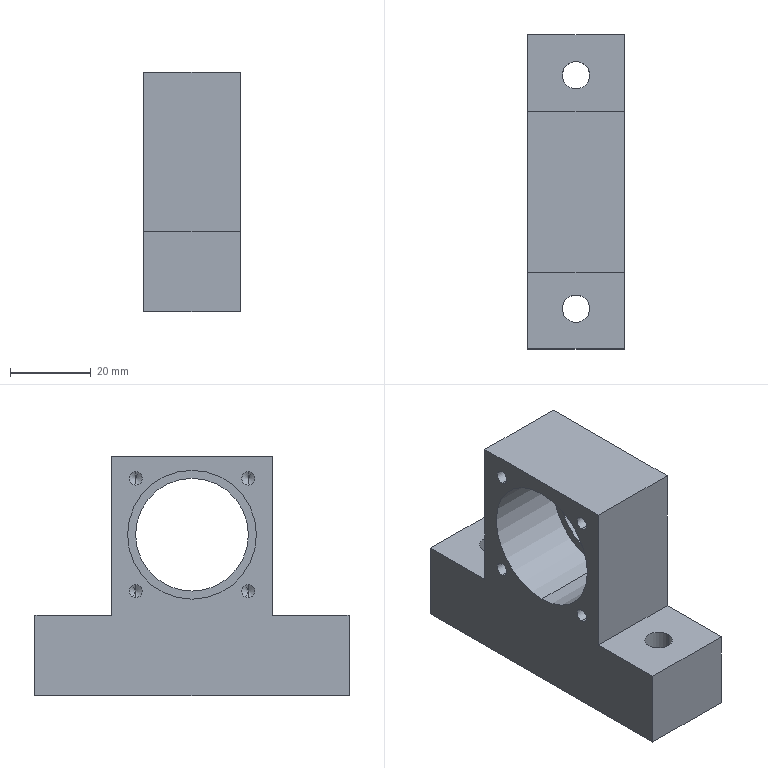Part | STEP file | PN_0080 main end seat | 1 solid | 35 faces | box 24 x 78 x 59.5 mm | volume 55003 mm3 | cylinder 16 | plane 11 | cone 8 | commonest cylinder face diameters 3.3 x8 6.8 x4 28 x2 32 x2